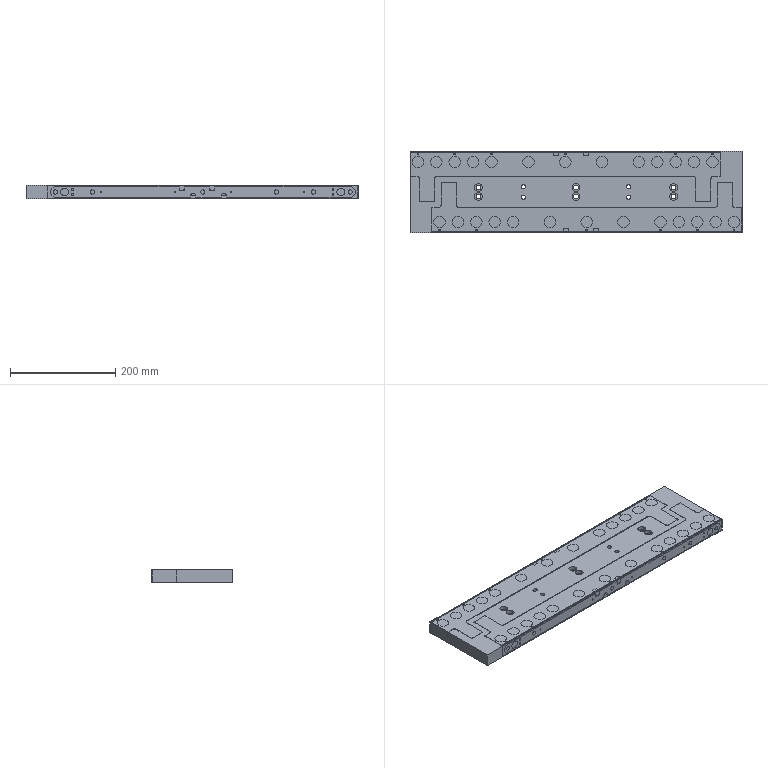Part | 13 solids | 742 faces | box 631 x 154 x 25 mm | volume 3776705 mm3 | cylinder 350 | plane 332 | cone 60 | commonest cylinder face diameters 22 x104 3.3 x64 16 x52 8 x36 15 x20 2.5 x16